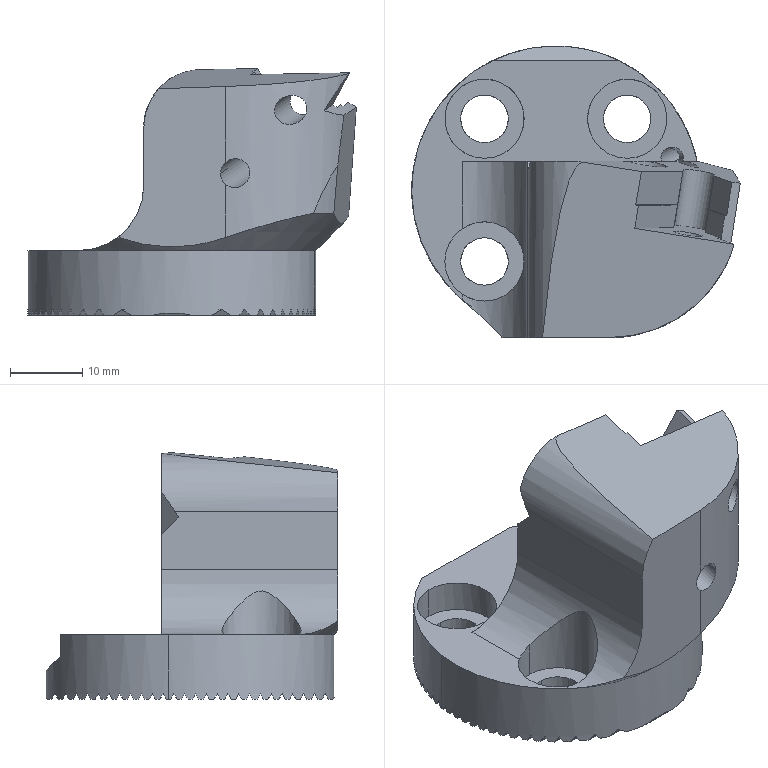Part | 1 solid | 215 faces | box 45.592 x 40.5 x 34.294 mm | volume 21555 mm3 | plane 176 | cylinder 35 | cone 4 | commonest cylinder face diameters 6.6 x6 11 x6 4 x5 1.5 x2 2.9 x2 3.3 x2